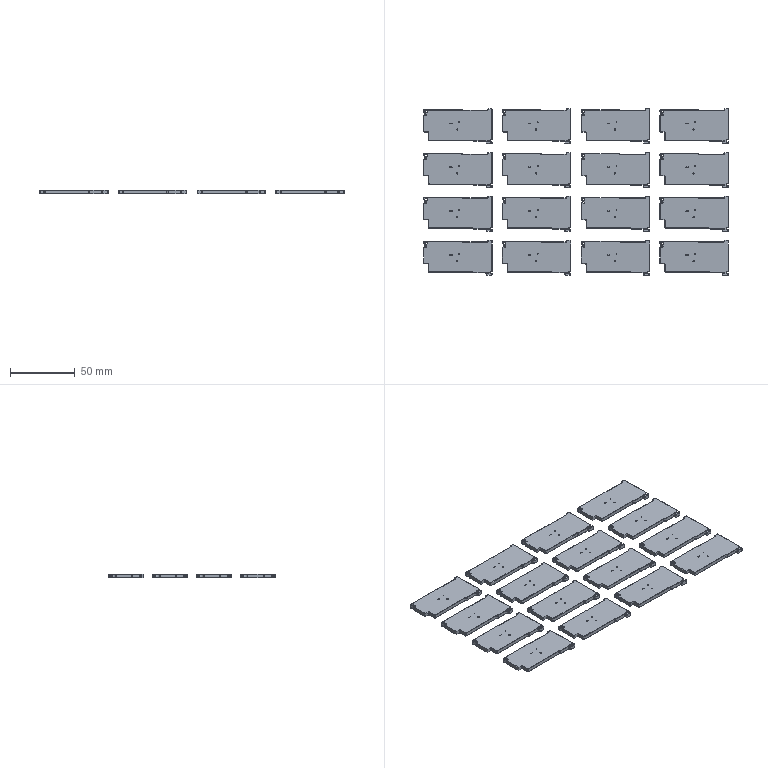Part | 16 solids | 1920 faces | box 236.046 x 129.136 x 3 mm | volume 59265 mm3 | plane 736 | cone 640 | cylinder 544 | commonest cylinder face diameters 1 x192 0.6 x96 1.1 x64 2 x64 1.8 x48 0.4 x32